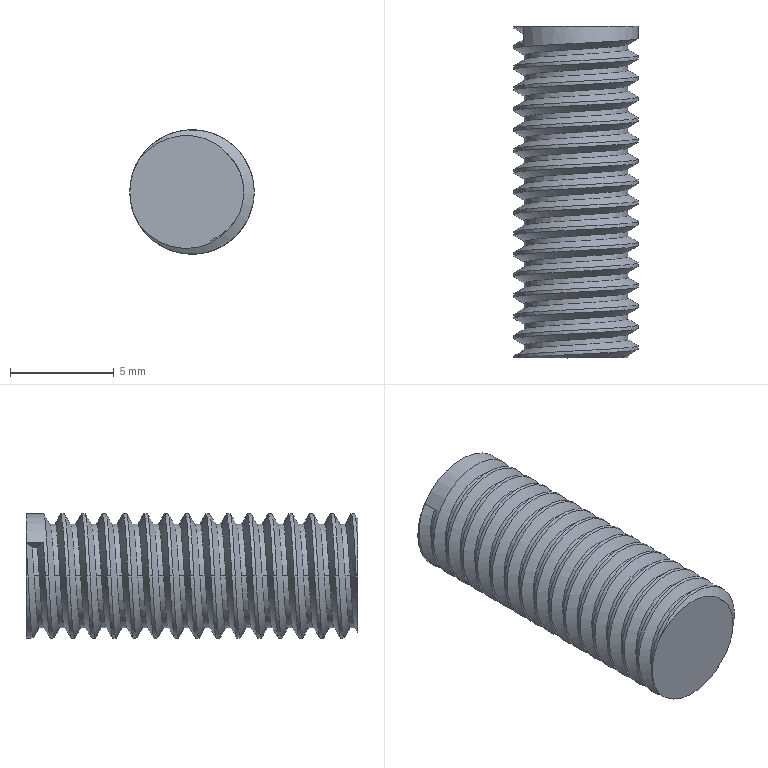Part | SolidWorks | features BaseBody 1 | 1 solid | 72 faces | box 6 x 16.008 x 6 mm | volume 378.104 mm3 | cylinder 67 | plane 3 | spline 2 | commonest cylinder face diameters 6 x34 5 x33